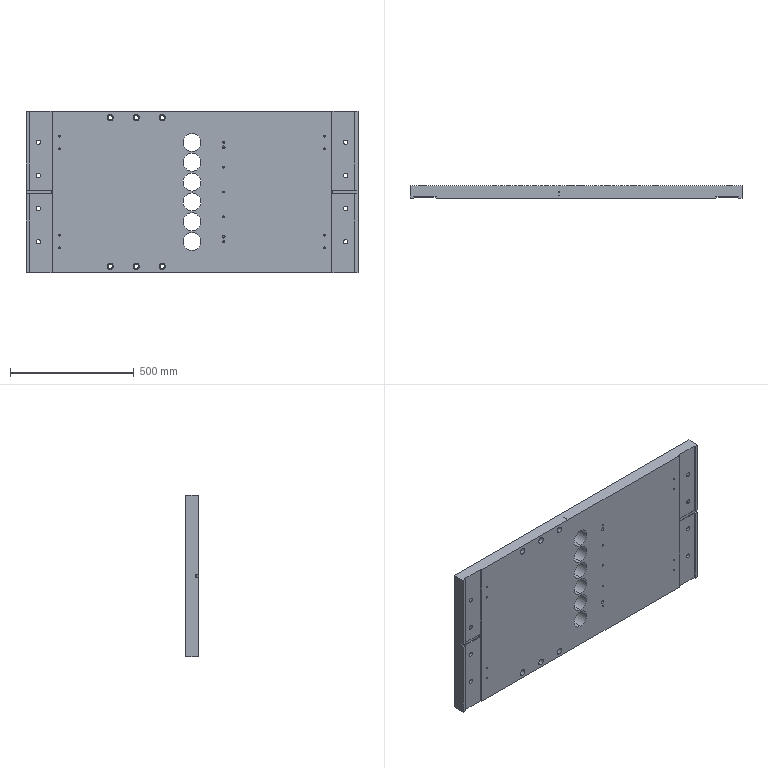Part | STEP file | forming top plate | 1 solid | 338 faces | box 1340 x 50 x 650 mm | volume 41398867 mm3 | cylinder 184 | cone 114 | plane 40 | commonest cylinder face diameters 6.8 x74 17.5 x28 26 x28 10.2 x16 72 x12 14 x10